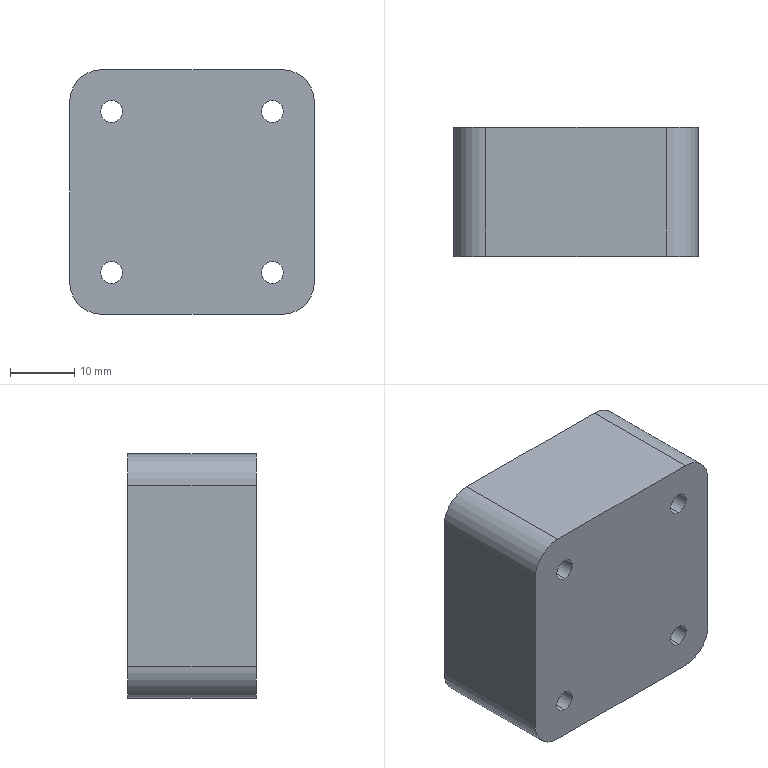Part | SolidWorks | features Extrusion 1, HoleWzd 1 | 1 solid | 30 faces | box 38 x 20 x 38 mm | volume 26957 mm3 | cylinder 20 | plane 10 | commonest cylinder face diameters 3.4 x8 6 x8 10 x4
STEP:
#1=CARTESIAN_POINT('',(-12.5,10.,-15.5));
#2=VERTEX_POINT('',#1);
#3=CARTESIAN_POINT('',(-12.5,10.,-9.5));
#4=VERTEX_POINT('',#3);
#5=CARTESIAN_POINT('',(-12.5,10.,-12.5));
#6=DIRECTION('',(0.,1.,0.));
#7=DIRECTION('',(0.,0.,1.));
#8=AXIS2_PLACEMENT_3D('',#5,#6,#7);
#9=CIRCLE('',#8,3.);
#10=EDGE_CURVE('',#2,#4,#9,.T.);
#11=ORIENTED_EDGE('',*,*,#10,.F.);
#12=CARTESIAN_POINT('',(-12.5,20.,-15.5));
#13=VERTEX_POINT('',#12);
#14=CARTESIAN_POINT('',(-12.5,20.,-15.5));
#15=DIRECTION('',(0.,1.,0.));
#16=VECTOR('',#15,1000.);
#17=LINE('',#14,#16);
#18=EDGE_CURVE('',#2,#13,#17,.T.);
#19=ORIENTED_EDGE('',*,*,#18,.T.);
#20=CARTESIAN_POINT('',(-12.5,20.,-9.5));
#21=VERTEX_POINT('',#20);
#22=CARTESIAN_POINT('',(-12.5,20.,-12.5));
#23=DIRECTION('',(0.,1.,0.));
#24=DIRECTION('',(0.,0.,1.));
#25=AXIS2_PLACEMENT_3D('',#22,#23,#24);
#26=CIRCLE('',#25,3.);
#27=EDGE_CURVE('',#13,#21,#26,.T.);
#28=ORIENTED_EDGE('',*,*,#27,.T.);
#29=CARTESIAN_POINT('',(-12.5,20.,-9.5));
#30=DIRECTION('',(0.,1.,0.));
#31=VECTOR('',#30,1000.);
#32=LINE('',#29,#31);
#33=EDGE_CURVE('',#4,#21,#32,.T.);
#34=ORIENTED_EDGE('',*,*,#33,.F.);
#35=EDGE_LOOP('',(#11,#19,#28,#34));
#36=FACE_OUTER_BOUND('',#35,.T.);
#37=CARTESIAN_POINT('',(-12.5,20.,-12.5));
#38=DIRECTION('',(0.,1.,0.));
#39=DIRECTION('',(0.,0.,1.));
#40=AXIS2_PLACEMENT_3D('',#37,#38,#39);
#41=CYLINDRICAL_SURFACE('',#40,3.);
#42=ADVANCED_FACE('',(#36),#41,.F.);
#43=CARTESIAN_POINT('',(-12.5,0.,-14.2));
#44=VERTEX_POINT('',#43);
#45=CARTESIAN_POINT('',(-12.5,0.,-10.8));
#46=VERTEX_POINT('',#45);
#47=CARTESIAN_POINT('',(-12.5,0.,-12.5));
#48=DIRECTION('',(0.,1.,0.));
#49=DIRECTION('',(0.,0.,1.));
#50=AXIS2_PLACEMENT_3D('',#47,#48,#49);
#51=CIRCLE('',#50,1.7);
#52=EDGE_CURVE('',#44,#46,#51,.T.);
#53=ORIENTED_EDGE('',*,*,#52,.F.);
#54=CARTESIAN_POINT('',(-12.5,10.,-14.2));
#55=VERTEX_POINT('',#54);
#56=CARTESIAN_POINT('',(-12.5,20.,-14.2));
#57=DIRECTION('',(0.,1.,0.));
#58=VECTOR('',#57,1000.);
#59=LINE('',#56,#58);
#60=EDGE_CURVE('',#44,#55,#59,.T.);
#61=ORIENTED_EDGE('',*,*,#60,.T.);
#62=CARTESIAN_POINT('',(-12.5,10.,-10.8));
#63=VERTEX_POINT('',#62);
#64=CARTESIAN_POINT('',(-12.5,10.,-12.5));
#65=DIRECTION('',(0.,1.,0.));
#66=DIRECTION('',(0.,0.,1.));
#67=AXIS2_PLACEMENT_3D('',#64,#65,#66);
#68=CIRCLE('',#67,1.7);
#69=EDGE_CURVE('',#55,#63,#68,.T.);
#70=ORIENTED_EDGE('',*,*,#69,.T.);
#71=CARTESIAN_POINT('',(-12.5,20.,-10.8));
#72=DIRECTION('',(0.,1.,0.));
#73=VECTOR('',#72,1000.);
#74=LINE('',#71,#73);
#75=EDGE_CURVE('',#46,#63,#74,.T.);
#76=ORIENTED_EDGE('',*,*,#75,.F.);
#77=EDGE_LOOP('',(#53,#61,#70,#76));
#78=FACE_OUTER_BOUND('',#77,.T.);
#79=CARTESIAN_POINT('',(-12.5,20.,-12.5));
#80=DIRECTION('',(0.,1.,0.));
#81=DIRECTION('',(0.,0.,1.));
#82=AXIS2_PLACEMENT_3D('',#79,#80,#81);
#83=CYLINDRICAL_SURFACE('',#82,1.7);
#84=ADVANCED_FACE('',(#78),#83,.F.);
#85=CARTESIAN_POINT('',(12.5,10.,-15.5));
#86=VERTEX_POINT('',#85);
#87=CARTESIAN_POINT('',(12.5,10.,-9.5));
#88=VERTEX_POINT('',#87);
#89=CARTESIAN_POINT('',(12.5,10.,-12.5));
#90=DIRECTION('',(0.,1.,0.));
#91=DIRECTION('',(0.,0.,1.));
#92=AXIS2_PLACEMENT_3D('',#89,#90,#91);
#93=CIRCLE('',#92,3.);
#94=EDGE_CURVE('',#86,#88,#93,.T.);
#95=ORIENTED_EDGE('',*,*,#94,.F.);
#96=CARTESIAN_POINT('',(12.5,20.,-15.5));
#97=VERTEX_POINT('',#96);
#98=CARTESIAN_POINT('',(12.5,20.,-15.5));
#99=DIRECTION('',(0.,1.,0.));
#100=VECTOR('',#99,1000.);
#101=LINE('',#98,#100);
#102=EDGE_CURVE('',#86,#97,#101,.T.);
#103=ORIENTED_EDGE('',*,*,#102,.T.);
#104=CARTESIAN_POINT('',(12.5,20.,-9.5));
#105=VERTEX_POINT('',#104);
#106=CARTESIAN_POINT('',(12.5,20.,-12.5));
#107=DIRECTION('',(0.,1.,0.));
#108=DIRECTION('',(0.,0.,1.));
#109=AXIS2_PLACEMENT_3D('',#106,#107,#108);
#110=CIRCLE('',#109,3.);
#111=EDGE_CURVE('',#97,#105,#110,.T.);
#112=ORIENTED_EDGE('',*,*,#111,.T.);
#113=CARTESIAN_POINT('',(12.5,20.,-9.5));
#114=DIRECTION('',(0.,1.,0.));
#115=VECTOR('',#114,1000.);
#116=LINE('',#113,#115);
#117=EDGE_CURVE('',#88,#105,#116,.T.);
#118=ORIENTED_EDGE('',*,*,#117,.F.);
#119=EDGE_LOOP('',(#95,#103,#112,#118));
#120=FACE_OUTER_BOUND('',#119,.T.);
#121=CARTESIAN_POINT('',(12.5,20.,-12.5));
#122=DIRECTION('',(0.,1.,0.));
#123=DIRECTION('',(0.,0.,1.));
#124=AXIS2_PLACEMENT_3D('',#121,#122,#123);
#125=CYLINDRICAL_SURFACE('',#124,3.);
#126=ADVANCED_FACE('',(#120),#125,.F.);
#127=CARTESIAN_POINT('',(12.5,0.,-14.2));
#128=VERTEX_POINT('',#127);
#129=CARTESIAN_POINT('',(12.5,0.,-10.8));
#130=VERTEX_POINT('',#129);
#131=CARTESIAN_POINT('',(12.5,0.,-12.5));
#132=DIRECTION('',(0.,1.,0.));
#133=DIRECTION('',(0.,0.,1.));
#134=AXIS2_PLACEMENT_3D('',#131,#132,#133);
#135=CIRCLE('',#134,1.7);
#136=EDGE_CURVE('',#128,#130,#135,.T.);
#137=ORIENTED_EDGE('',*,*,#136,.F.);
#138=CARTESIAN_POINT('',(12.5,10.,-14.2));
#139=VERTEX_POINT('',#138);
#140=CARTESIAN_POINT('',(12.5,20.,-14.2));
#141=DIRECTION('',(0.,1.,0.));
#142=VECTOR('',#141,1000.);
#143=LINE('',#140,#142);
#144=EDGE_CURVE('',#128,#139,#143,.T.);
#145=ORIENTED_EDGE('',*,*,#144,.T.);
#146=CARTESIAN_POINT('',(12.5,10.,-10.8));
#147=VERTEX_POINT('',#146);
#148=CARTESIAN_POINT('',(12.5,10.,-12.5));
#149=DIRECTION('',(0.,1.,0.));
#150=DIRECTION('',(0.,0.,1.));
#151=AXIS2_PLACEMENT_3D('',#148,#149,#150);
#152=CIRCLE('',#151,1.7);
#153=EDGE_CURVE('',#139,#147,#152,.T.);
#154=ORIENTED_EDGE('',*,*,#153,.T.);
#155=CARTESIAN_POINT('',(12.5,20.,-10.8));
#156=DIRECTION('',(0.,1.,0.));
#157=VECTOR('',#156,1000.);
#158=LINE('',#155,#157);
#159=EDGE_CURVE('',#130,#147,#158,.T.);
#160=ORIENTED_EDGE('',*,*,#159,.F.);
#161=EDGE_LOOP('',(#137,#145,#154,#160));
#162=FACE_OUTER_BOUND('',#161,.T.);
#163=CARTESIAN_POINT('',(12.5,20.,-12.5));
#164=DIRECTION('',(0.,1.,0.));
#165=DIRECTION('',(0.,0.,1.));
#166=AXIS2_PLACEMENT_3D('',#163,#164,#165);
#167=CYLINDRICAL_SURFACE('',#166,1.7);
#168=ADVANCED_FACE('',(#162),#167,.F.);
#169=CARTESIAN_POINT('',(12.5,10.,9.5));
#170=VERTEX_POINT('',#169);
#171=CARTESIAN_POINT('',(12.5,10.,15.5));
#172=VERTEX_POINT('',#171);
#173=CARTESIAN_POINT('',(12.5,10.,12.5));
#174=DIRECTION('',(0.,1.,0.));
#175=DIRECTION('',(0.,0.,1.));
#176=AXIS2_PLACEMENT_3D('',#173,#174,#175);
#177=CIRCLE('',#176,3.);
#178=EDGE_CURVE('',#170,#172,#177,.T.);
#179=ORIENTED_EDGE('',*,*,#178,.F.);
#180=CARTESIAN_POINT('',(12.5,20.,9.5));
#181=VERTEX_POINT('',#180);
#182=CARTESIAN_POINT('',(12.5,20.,9.5));
#183=DIRECTION('',(0.,1.,0.));
#184=VECTOR('',#183,1000.);
#185=LINE('',#182,#184);
#186=EDGE_CURVE('',#170,#181,#185,.T.);
#187=ORIENTED_EDGE('',*,*,#186,.T.);
#188=CARTESIAN_POINT('',(12.5,20.,15.5));
#189=VERTEX_POINT('',#188);
#190=CARTESIAN_POINT('',(12.5,20.,12.5));
#191=DIRECTION('',(0.,1.,0.));
#192=DIRECTION('',(0.,0.,1.));
#193=AXIS2_PLACEMENT_3D('',#190,#191,#192);
#194=CIRCLE('',#193,3.);
#195=EDGE_CURVE('',#181,#189,#194,.T.);
#196=ORIENTED_EDGE('',*,*,#195,.T.);
#197=CARTESIAN_POINT('',(12.5,20.,15.5));
#198=DIRECTION('',(0.,1.,0.));
#199=VECTOR('',#198,1000.);
#200=LINE('',#197,#199);
#201=EDGE_CURVE('',#172,#189,#200,.T.);
#202=ORIENTED_EDGE('',*,*,#201,.F.);
#203=EDGE_LOOP('',(#179,#187,#196,#202));
#204=FACE_OUTER_BOUND('',#203,.T.);
#205=CARTESIAN_POINT('',(12.5,20.,12.5));
#206=DIRECTION('',(0.,1.,0.));
#207=DIRECTION('',(0.,0.,1.));
#208=AXIS2_PLACEMENT_3D('',#205,#206,#207);
#209=CYLINDRICAL_SURFACE('',#208,3.);
#210=ADVANCED_FACE('',(#204),#209,.F.);
#211=CARTESIAN_POINT('',(12.5,0.,10.8));
#212=VERTEX_POINT('',#211);
#213=CARTESIAN_POINT('',(12.5,0.,14.2));
#214=VERTEX_POINT('',#213);
#215=CARTESIAN_POINT('',(12.5,0.,12.5));
#216=DIRECTION('',(0.,1.,0.));
#217=DIRECTION('',(0.,0.,1.));
#218=AXIS2_PLACEMENT_3D('',#215,#216,#217);
#219=CIRCLE('',#218,1.7);
#220=EDGE_CURVE('',#212,#214,#219,.T.);
#221=ORIENTED_EDGE('',*,*,#220,.F.);
#222=CARTESIAN_POINT('',(12.5,10.,10.8));
#223=VERTEX_POINT('',#222);
#224=CARTESIAN_POINT('',(12.5,20.,10.8));
#225=DIRECTION('',(0.,1.,0.));
#226=VECTOR('',#225,1000.);
#227=LINE('',#224,#226);
#228=EDGE_CURVE('',#212,#223,#227,.T.);
#229=ORIENTED_EDGE('',*,*,#228,.T.);
#230=CARTESIAN_POINT('',(12.5,10.,14.2));
#231=VERTEX_POINT('',#230);
#232=CARTESIAN_POINT('',(12.5,10.,12.5));
#233=DIRECTION('',(0.,1.,0.));
#234=DIRECTION('',(0.,0.,1.));
#235=AXIS2_PLACEMENT_3D('',#232,#233,#234);
#236=CIRCLE('',#235,1.7);
#237=EDGE_CURVE('',#223,#231,#236,.T.);
#238=ORIENTED_EDGE('',*,*,#237,.T.);
#239=CARTESIAN_POINT('',(12.5,20.,14.2));
#240=DIRECTION('',(0.,1.,0.));
#241=VECTOR('',#240,1000.);
#242=LINE('',#239,#241);
#243=EDGE_CURVE('',#214,#231,#242,.T.);
#244=ORIENTED_EDGE('',*,*,#243,.F.);
#245=EDGE_LOOP('',(#221,#229,#238,#244));
#246=FACE_OUTER_BOUND('',#245,.T.);
#247=CARTESIAN_POINT('',(12.5,20.,12.5));
#248=DIRECTION('',(0.,1.,0.));
#249=DIRECTION('',(0.,0.,1.));
#250=AXIS2_PLACEMENT_3D('',#247,#248,#249);
#251=CYLINDRICAL_SURFACE('',#250,1.7);
#252=ADVANCED_FACE('',(#246),#251,.F.);
#253=CARTESIAN_POINT('',(-12.5,10.,9.5));
#254=VERTEX_POINT('',#253);
#255=CARTESIAN_POINT('',(-12.5,10.,15.5));
#256=VERTEX_POINT('',#255);
#257=CARTESIAN_POINT('',(-12.5,10.,12.5));
#258=DIRECTION('',(0.,1.,0.));
#259=DIRECTION('',(0.,0.,1.));
#260=AXIS2_PLACEMENT_3D('',#257,#258,#259);
#261=CIRCLE('',#260,3.);
#262=EDGE_CURVE('',#254,#256,#261,.T.);
#263=ORIENTED_EDGE('',*,*,#262,.F.);
#264=CARTESIAN_POINT('',(-12.5,20.,9.5));
#265=VERTEX_POINT('',#264);
#266=CARTESIAN_POINT('',(-12.5,20.,9.5));
#267=DIRECTION('',(0.,1.,0.));
#268=VECTOR('',#267,1000.);
#269=LINE('',#266,#268);
#270=EDGE_CURVE('',#254,#265,#269,.T.);
#271=ORIENTED_EDGE('',*,*,#270,.T.);
#272=CARTESIAN_POINT('',(-12.5,20.,15.5));
#273=VERTEX_POINT('',#272);
#274=CARTESIAN_POINT('',(-12.5,20.,12.5));
#275=DIRECTION('',(0.,1.,0.));
#276=DIRECTION('',(0.,0.,1.));
#277=AXIS2_PLACEMENT_3D('',#274,#275,#276);
#278=CIRCLE('',#277,3.);
#279=EDGE_CURVE('',#265,#273,#278,.T.);
#280=ORIENTED_EDGE('',*,*,#279,.T.);
#281=CARTESIAN_POINT('',(-12.5,20.,15.5));
#282=DIRECTION('',(0.,1.,0.));
#283=VECTOR('',#282,1000.);
#284=LINE('',#281,#283);
#285=EDGE_CURVE('',#256,#273,#284,.T.);
#286=ORIENTED_EDGE('',*,*,#285,.F.);
#287=EDGE_LOOP('',(#263,#271,#280,#286));
#288=FACE_OUTER_BOUND('',#287,.T.);
#289=CARTESIAN_POINT('',(-12.5,20.,12.5));
#290=DIRECTION('',(0.,1.,0.));
#291=DIRECTION('',(0.,0.,1.));
#292=AXIS2_PLACEMENT_3D('',#289,#290,#291);
#293=CYLINDRICAL_SURFACE('',#292,3.);
#294=ADVANCED_FACE('',(#288),#293,.F.);
#295=CARTESIAN_POINT('',(-12.5,0.,10.8));
#296=VERTEX_POINT('',#295);
#297=CARTESIAN_POINT('',(-12.5,0.,14.2));
#298=VERTEX_POINT('',#297);
#299=CARTESIAN_POINT('',(-12.5,0.,12.5));
#300=DIRECTION('',(0.,1.,0.));
#301=DIRECTION('',(0.,0.,1.));
#302=AXIS2_PLACEMENT_3D('',#299,#300,#301);
#303=CIRCLE('',#302,1.7);
#304=EDGE_CURVE('',#296,#298,#303,.T.);
#305=ORIENTED_EDGE('',*,*,#304,.F.);
#306=CARTESIAN_POINT('',(-12.5,10.,10.8));
#307=VERTEX_POINT('',#306);
#308=CARTESIAN_POINT('',(-12.5,20.,10.8));
#309=DIRECTION('',(0.,1.,0.));
#310=VECTOR('',#309,1000.);
#311=LINE('',#308,#310);
#312=EDGE_CURVE('',#296,#307,#311,.T.);
#313=ORIENTED_EDGE('',*,*,#312,.T.);
#314=CARTESIAN_POINT('',(-12.5,10.,14.2));
#315=VERTEX_POINT('',#314);
#316=CARTESIAN_POINT('',(-12.5,10.,12.5));
#317=DIRECTION('',(0.,1.,0.));
#318=DIRECTION('',(0.,0.,1.));
#319=AXIS2_PLACEMENT_3D('',#316,#317,#318);
#320=CIRCLE('',#319,1.7);
#321=EDGE_CURVE('',#307,#315,#320,.T.);
#322=ORIENTED_EDGE('',*,*,#321,.T.);
#323=CARTESIAN_POINT('',(-12.5,20.,14.2));
#324=DIRECTION('',(0.,1.,0.));
#325=VECTOR('',#324,1000.);
#326=LINE('',#323,#325);
#327=EDGE_CURVE('',#298,#315,#326,.T.);
#328=ORIENTED_EDGE('',*,*,#327,.F.);
#329=EDGE_LOOP('',(#305,#313,#322,#328));
#330=FACE_OUTER_BOUND('',#329,.T.);
#331=CARTESIAN_POINT('',(-12.5,20.,12.5));
#332=DIRECTION('',(0.,1.,0.));
#333=DIRECTION('',(0.,0.,1.));
#334=AXIS2_PLACEMENT_3D('',#331,#332,#333);
#335=CYLINDRICAL_SURFACE('',#334,1.7);
#336=ADVANCED_FACE('',(#330),#335,.F.);
#337=CARTESIAN_POINT('',(19.,0.,-14.));
#338=VERTEX_POINT('',#337);
#339=CARTESIAN_POINT('',(14.,0.,-19.));
#340=VERTEX_POINT('',#339);
#341=CARTESIAN_POINT('',(14.,0.,-14.));
#342=DIRECTION('',(0.,1.,0.));
#343=DIRECTION('',(0.,0.,-1.));
#344=AXIS2_PLACEMENT_3D('',#341,#342,#343);
#345=CIRCLE('',#344,5.);
#346=EDGE_CURVE('',#338,#340,#345,.T.);
#347=ORIENTED_EDGE('',*,*,#346,.T.);
#348=CARTESIAN_POINT('',(14.,20.,-19.));
#349=VERTEX_POINT('',#348);
#350=CARTESIAN_POINT('',(14.,20.,-19.));
#351=DIRECTION('',(0.,-1.,0.));
#352=VECTOR('',#351,1000.);
#353=LINE('',#350,#352);
#354=EDGE_CURVE('',#349,#340,#353,.T.);
#355=ORIENTED_EDGE('',*,*,#354,.F.);
#356=CARTESIAN_POINT('',(19.,20.,-14.));
#357=VERTEX_POINT('',#356);
#358=CARTESIAN_POINT('',(14.,20.,-14.));
#359=DIRECTION('',(0.,1.,0.));
#360=DIRECTION('',(0.,0.,-1.));
#361=AXIS2_PLACEMENT_3D('',#358,#359,#360);
#362=CIRCLE('',#361,5.);
#363=EDGE_CURVE('',#357,#349,#362,.T.);
#364=ORIENTED_EDGE('',*,*,#363,.F.);
#365=CARTESIAN_POINT('',(19.,20.,-14.));
#366=DIRECTION('',(0.,-1.,0.));
#367=VECTOR('',#366,1000.);
#368=LINE('',#365,#367);
#369=EDGE_CURVE('',#357,#338,#368,.T.);
#370=ORIENTED_EDGE('',*,*,#369,.T.);
#371=EDGE_LOOP('',(#347,#355,#364,#370));
#372=FACE_OUTER_BOUND('',#371,.T.);
#373=CARTESIAN_POINT('',(14.,20.,-14.));
#374=DIRECTION('',(0.,-1.,0.));
#375=DIRECTION('',(0.,0.,-1.));
#376=AXIS2_PLACEMENT_3D('',#373,#374,#375);
#377=CYLINDRICAL_SURFACE('',#376,5.);
#378=ADVANCED_FACE('',(#372),#377,.T.);
#379=CARTESIAN_POINT('',(-14.,0.,-19.));
#380=VERTEX_POINT('',#379);
#381=CARTESIAN_POINT('',(-14.,0.,-19.));
#382=DIRECTION('',(-1.,0.,0.));
#383=VECTOR('',#382,1000.);
#384=LINE('',#381,#383);
#385=EDGE_CURVE('',#340,#380,#384,.T.);
#386=ORIENTED_EDGE('',*,*,#385,.T.);
#387=CARTESIAN_POINT('',(-14.,20.,-19.));
#388=VERTEX_POINT('',#387);
#389=CARTESIAN_POINT('',(-14.,20.,-19.));
#390=DIRECTION('',(0.,-1.,0.));
#391=VECTOR('',#390,1000.);
#392=LINE('',#389,#391);
#393=EDGE_CURVE('',#388,#380,#392,.T.);
#394=ORIENTED_EDGE('',*,*,#393,.F.);
#395=CARTESIAN_POINT('',(-14.,20.,-19.));
#396=DIRECTION('',(-1.,0.,0.));
#397=VECTOR('',#396,1000.);
#398=LINE('',#395,#397);
#399=EDGE_CURVE('',#349,#388,#398,.T.);
#400=ORIENTED_EDGE('',*,*,#399,.F.);
#401=ORIENTED_EDGE('',*,*,#354,.T.);
#402=EDGE_LOOP('',(#386,#394,#400,#401));
#403=FACE_OUTER_BOUND('',#402,.T.);
#404=CARTESIAN_POINT('',(-14.,20.,-19.));
#405=DIRECTION('',(0.,0.,1.));
#406=DIRECTION('',(1.,0.,0.));
#407=AXIS2_PLACEMENT_3D('',#404,#405,#406);
#408=PLANE('',#407);
#409=ADVANCED_FACE('',(#403),#408,.F.);
#410=CARTESIAN_POINT('',(-19.,0.,-14.));
#411=VERTEX_POINT('',#410);
#412=CARTESIAN_POINT('',(-14.,0.,-14.));
#413=DIRECTION('',(0.,1.,0.));
#414=DIRECTION('',(0.,0.,1.));
#415=AXIS2_PLACEMENT_3D('',#412,#413,#414);
#416=CIRCLE('',#415,5.);
#417=EDGE_CURVE('',#380,#411,#416,.T.);
#418=ORIENTED_EDGE('',*,*,#417,.T.);
#419=CARTESIAN_POINT('',(-19.,20.,-14.));
#420=VERTEX_POINT('',#419);
#421=CARTESIAN_POINT('',(-19.,20.,-14.));
#422=DIRECTION('',(0.,-1.,0.));
#423=VECTOR('',#422,1000.);
#424=LINE('',#421,#423);
#425=EDGE_CURVE('',#420,#411,#424,.T.);
#426=ORIENTED_EDGE('',*,*,#425,.F.);
#427=CARTESIAN_POINT('',(-14.,20.,-14.));
#428=DIRECTION('',(0.,1.,0.));
#429=DIRECTION('',(0.,0.,1.));
#430=AXIS2_PLACEMENT_3D('',#427,#428,#429);
#431=CIRCLE('',#430,5.);
#432=EDGE_CURVE('',#388,#420,#431,.T.);
#433=ORIENTED_EDGE('',*,*,#432,.F.);
#434=ORIENTED_EDGE('',*,*,#393,.T.);
#435=EDGE_LOOP('',(#418,#426,#433,#434));
#436=FACE_OUTER_BOUND('',#435,.T.);
#437=CARTESIAN_POINT('',(-14.,20.,-14.));
#438=DIRECTION('',(0.,-1.,0.));
#439=DIRECTION('',(0.,0.,-1.));
#440=AXIS2_PLACEMENT_3D('',#437,#438,#439);
#441=CYLINDRICAL_SURFACE('',#440,5.);
#442=ADVANCED_FACE('',(#436),#441,.T.);
#443=CARTESIAN_POINT('',(-19.,0.,14.));
#444=VERTEX_POINT('',#443);
#445=CARTESIAN_POINT('',(-19.,0.,-14.));
#446=DIRECTION('',(0.,0.,1.));
#447=VECTOR('',#446,1000.);
#448=LINE('',#445,#447);
#449=EDGE_CURVE('',#411,#444,#448,.T.);
#450=ORIENTED_EDGE('',*,*,#449,.T.);
#451=CARTESIAN_POINT('',(-19.,20.,14.));
#452=VERTEX_POINT('',#451);
#453=CARTESIAN_POINT('',(-19.,20.,14.));
#454=DIRECTION('',(0.,-1.,0.));
#455=VECTOR('',#454,1000.);
#456=LINE('',#453,#455);
#457=EDGE_CURVE('',#452,#444,#456,.T.);
#458=ORIENTED_EDGE('',*,*,#457,.F.);
#459=CARTESIAN_POINT('',(-19.,20.,-14.));
#460=DIRECTION('',(0.,0.,1.));
#461=VECTOR('',#460,1000.);
#462=LINE('',#459,#461);
#463=EDGE_CURVE('',#420,#452,#462,.T.);
#464=ORIENTED_EDGE('',*,*,#463,.F.);
#465=ORIENTED_EDGE('',*,*,#425,.T.);
#466=EDGE_LOOP('',(#450,#458,#464,#465));
#467=FACE_OUTER_BOUND('',#466,.T.);
#468=CARTESIAN_POINT('',(-19.,20.,-14.));
#469=DIRECTION('',(1.,0.,0.));
#470=DIRECTION('',(0.,0.,-1.));
#471=AXIS2_PLACEMENT_3D('',#468,#469,#470);
#472=PLANE('',#471);
#473=ADVANCED_FACE('',(#467),#472,.F.);
#474=CARTESIAN_POINT('',(-14.,0.,19.));
#475=VERTEX_POINT('',#474);
#476=CARTESIAN_POINT('',(-14.,0.,14.));
#477=DIRECTION('',(0.,1.,0.));
#478=DIRECTION('',(0.,0.,1.));
#479=AXIS2_PLACEMENT_3D('',#476,#477,#478);
#480=CIRCLE('',#479,5.);
#481=EDGE_CURVE('',#444,#475,#480,.T.);
#482=ORIENTED_EDGE('',*,*,#481,.T.);
#483=CARTESIAN_POINT('',(-14.,20.,19.));
#484=VERTEX_POINT('',#483);
#485=CARTESIAN_POINT('',(-14.,20.,19.));
#486=DIRECTION('',(0.,-1.,0.));
#487=VECTOR('',#486,1000.);
#488=LINE('',#485,#487);
#489=EDGE_CURVE('',#484,#475,#488,.T.);
#490=ORIENTED_EDGE('',*,*,#489,.F.);
#491=CARTESIAN_POINT('',(-14.,20.,14.));
#492=DIRECTION('',(0.,1.,0.));
#493=DIRECTION('',(0.,0.,1.));
#494=AXIS2_PLACEMENT_3D('',#491,#492,#493);
#495=CIRCLE('',#494,5.);
#496=EDGE_CURVE('',#452,#484,#495,.T.);
#497=ORIENTED_EDGE('',*,*,#496,.F.);
#498=ORIENTED_EDGE('',*,*,#457,.T.);
#499=EDGE_LOOP('',(#482,#490,#497,#498));
#500=FACE_OUTER_BOUND('',#499,.T.);
#501=CARTESIAN_POINT('',(-14.,20.,14.));
#502=DIRECTION('',(0.,-1.,0.));
#503=DIRECTION('',(0.,0.,-1.));
#504=AXIS2_PLACEMENT_3D('',#501,#502,#503);
#505=CYLINDRICAL_SURFACE('',#504,5.);
#506=ADVANCED_FACE('',(#500),#505,.T.);
#507=CARTESIAN_POINT('',(14.,0.,19.));
#508=VERTEX_POINT('',#507);
#509=CARTESIAN_POINT('',(-14.,0.,19.));
#510=DIRECTION('',(1.,0.,0.));
#511=VECTOR('',#510,1000.);
#512=LINE('',#509,#511);
#513=EDGE_CURVE('',#475,#508,#512,.T.);
#514=ORIENTED_EDGE('',*,*,#513,.T.);
#515=CARTESIAN_POINT('',(14.,20.,19.));
#516=VERTEX_POINT('',#515);
#517=CARTESIAN_POINT('',(14.,20.,19.));
#518=DIRECTION('',(0.,-1.,0.));
#519=VECTOR('',#518,1000.);
#520=LINE('',#517,#519);
#521=EDGE_CURVE('',#516,#508,#520,.T.);
#522=ORIENTED_EDGE('',*,*,#521,.F.);
#523=CARTESIAN_POINT('',(-14.,20.,19.));
#524=DIRECTION('',(1.,0.,0.));
#525=VECTOR('',#524,1000.);
#526=LINE('',#523,#525);
#527=EDGE_CURVE('',#484,#516,#526,.T.);
#528=ORIENTED_EDGE('',*,*,#527,.F.);
#529=ORIENTED_EDGE('',*,*,#489,.T.);
#530=EDGE_LOOP('',(#514,#522,#528,#529));
#531=FACE_OUTER_BOUND('',#530,.T.);
#532=CARTESIAN_POINT('',(-14.,20.,19.));
#533=DIRECTION('',(0.,0.,-1.));
#534=DIRECTION('',(-1.,0.,0.));
#535=AXIS2_PLACEMENT_3D('',#532,#533,#534);
#536=PLANE('',#535);
#537=ADVANCED_FACE('',(#531),#536,.F.);
#538=CARTESIAN_POINT('',(19.,0.,14.));
#539=VERTEX_POINT('',#538);
#540=CARTESIAN_POINT('',(14.,0.,14.));
#541=DIRECTION('',(0.,1.,0.));
#542=DIRECTION('',(0.,0.,1.));
#543=AXIS2_PLACEMENT_3D('',#540,#541,#542);
#544=CIRCLE('',#543,5.);
#545=EDGE_CURVE('',#508,#539,#544,.T.);
#546=ORIENTED_EDGE('',*,*,#545,.T.);
#547=CARTESIAN_POINT('',(19.,20.,14.));
#548=VERTEX_POINT('',#547);
#549=CARTESIAN_POINT('',(19.,20.,14.));
#550=DIRECTION('',(0.,-1.,0.));
#551=VECTOR('',#550,1000.);
#552=LINE('',#549,#551);
#553=EDGE_CURVE('',#548,#539,#552,.T.);
#554=ORIENTED_EDGE('',*,*,#553,.F.);
#555=CARTESIAN_POINT('',(14.,20.,14.));
#556=DIRECTION('',(0.,1.,0.));
#557=DIRECTION('',(0.,0.,1.));
#558=AXIS2_PLACEMENT_3D('',#555,#556,#557);
#559=CIRCLE('',#558,5.);
#560=EDGE_CURVE('',#516,#548,#559,.T.);
#561=ORIENTED_EDGE('',*,*,#560,.F.);
#562=ORIENTED_EDGE('',*,*,#521,.T.);
#563=EDGE_LOOP('',(#546,#554,#561,#562));
#564=FACE_OUTER_BOUND('',#563,.T.);
#565=CARTESIAN_POINT('',(14.,20.,14.));
#566=DIRECTION('',(0.,-1.,0.));
#567=DIRECTION('',(0.,0.,-1.));
#568=AXIS2_PLACEMENT_3D('',#565,#566,#567);
#569=CYLINDRICAL_SURFACE('',#568,5.);
#570=ADVANCED_FACE('',(#564),#569,.T.);
#571=CARTESIAN_POINT('',(19.,0.,-14.));
#572=DIRECTION('',(0.,0.,-1.));
#573=VECTOR('',#572,1000.);
#574=LINE('',#571,#573);
#575=EDGE_CURVE('',#539,#338,#574,.T.);
#576=ORIENTED_EDGE('',*,*,#575,.T.);
#577=ORIENTED_EDGE('',*,*,#369,.F.);
#578=CARTESIAN_POINT('',(19.,20.,-14.));
#579=DIRECTION('',(0.,0.,-1.));
#580=VECTOR('',#579,1000.);
#581=LINE('',#578,#580);
#582=EDGE_CURVE('',#548,#357,#581,.T.);
#583=ORIENTED_EDGE('',*,*,#582,.F.);
#584=ORIENTED_EDGE('',*,*,#553,.T.);
#585=EDGE_LOOP('',(#576,#577,#583,#584));
#586=FACE_OUTER_BOUND('',#585,.T.);
#587=CARTESIAN_POINT('',(19.,20.,-14.));
#588=DIRECTION('',(-1.,0.,0.));
#589=DIRECTION('',(0.,0.,1.));
#590=AXIS2_PLACEMENT_3D('',#587,#588,#589);
#591=PLANE('',#590);
#592=ADVANCED_FACE('',(#586),#591,.F.);
#593=CARTESIAN_POINT('',(-12.5,20.,-12.5));
#594=DIRECTION('',(0.,1.,0.));
#595=DIRECTION('',(0.,0.,1.));
#596=AXIS2_PLACEMENT_3D('',#593,#594,#595);
#597=CIRCLE('',#596,3.);
#598=EDGE_CURVE('',#21,#13,#597,.T.);
#599=ORIENTED_EDGE('',*,*,#598,.F.);
#600=ORIENTED_EDGE('',*,*,#27,.F.);
#601=EDGE_LOOP('',(#599,#600));
#602=FACE_BOUND('',#601,.T.);
#603=CARTESIAN_POINT('',(12.5,20.,-12.5));
#604=DIRECTION('',(0.,1.,0.));
#605=DIRECTION('',(0.,0.,1.));
#606=AXIS2_PLACEMENT_3D('',#603,#604,#605);
#607=CIRCLE('',#606,3.);
#608=EDGE_CURVE('',#105,#97,#607,.T.);
#609=ORIENTED_EDGE('',*,*,#608,.F.);
#610=ORIENTED_EDGE('',*,*,#111,.F.);
#611=EDGE_LOOP('',(#609,#610));
#612=FACE_BOUND('',#611,.T.);
#613=CARTESIAN_POINT('',(12.5,20.,12.5));
#614=DIRECTION('',(0.,1.,0.));
#615=DIRECTION('',(0.,0.,1.));
#616=AXIS2_PLACEMENT_3D('',#613,#614,#615);
#617=CIRCLE('',#616,3.);
#618=EDGE_CURVE('',#189,#181,#617,.T.);
#619=ORIENTED_EDGE('',*,*,#618,.F.);
#620=ORIENTED_EDGE('',*,*,#195,.F.);
#621=EDGE_LOOP('',(#619,#620));
#622=FACE_BOUND('',#621,.T.);
#623=CARTESIAN_POINT('',(-12.5,20.,12.5));
#624=DIRECTION('',(0.,1.,0.));
#625=DIRECTION('',(0.,0.,1.));
#626=AXIS2_PLACEMENT_3D('',#623,#624,#625);
#627=CIRCLE('',#626,3.);
#628=EDGE_CURVE('',#273,#265,#627,.T.);
#629=ORIENTED_EDGE('',*,*,#628,.F.);
#630=ORIENTED_EDGE('',*,*,#279,.F.);
#631=EDGE_LOOP('',(#629,#630));
#632=FACE_BOUND('',#631,.T.);
#633=ORIENTED_EDGE('',*,*,#363,.T.);
#634=ORIENTED_EDGE('',*,*,#399,.T.);
#635=ORIENTED_EDGE('',*,*,#432,.T.);
#636=ORIENTED_EDGE('',*,*,#463,.T.);
#637=ORIENTED_EDGE('',*,*,#496,.T.);
#638=ORIENTED_EDGE('',*,*,#527,.T.);
#639=ORIENTED_EDGE('',*,*,#560,.T.);
#640=ORIENTED_EDGE('',*,*,#582,.T.);
#641=EDGE_LOOP('',(#633,#634,#635,#636,#637,#638,#639,#640));
#642=FACE_OUTER_BOUND('',#641,.T.);
#643=CARTESIAN_POINT('',(14.,20.,-14.));
#644=DIRECTION('',(0.,-1.,0.));
#645=DIRECTION('',(0.,0.,-1.));
#646=AXIS2_PLACEMENT_3D('',#643,#644,#645);
#647=PLANE('',#646);
#648=ADVANCED_FACE('',(#602,#612,#622,#632,#642),#647,.F.);
#649=CARTESIAN_POINT('',(-12.5,0.,-12.5));
#650=DIRECTION('',(0.,1.,0.));
#651=DIRECTION('',(0.,0.,1.));
#652=AXIS2_PLACEMENT_3D('',#649,#650,#651);
#653=CIRCLE('',#652,1.7);
#654=EDGE_CURVE('',#46,#44,#653,.T.);
#655=ORIENTED_EDGE('',*,*,#654,.T.);
#656=ORIENTED_EDGE('',*,*,#52,.T.);
#657=EDGE_LOOP('',(#655,#656));
#658=FACE_BOUND('',#657,.T.);
#659=CARTESIAN_POINT('',(12.5,0.,-12.5));
#660=DIRECTION('',(0.,1.,0.));
#661=DIRECTION('',(0.,0.,1.));
#662=AXIS2_PLACEMENT_3D('',#659,#660,#661);
#663=CIRCLE('',#662,1.7);
#664=EDGE_CURVE('',#130,#128,#663,.T.);
#665=ORIENTED_EDGE('',*,*,#664,.T.);
#666=ORIENTED_EDGE('',*,*,#136,.T.);
#667=EDGE_LOOP('',(#665,#666));
#668=FACE_BOUND('',#667,.T.);
#669=CARTESIAN_POINT('',(12.5,0.,12.5));
#670=DIRECTION('',(0.,1.,0.));
#671=DIRECTION('',(0.,0.,1.));
#672=AXIS2_PLACEMENT_3D('',#669,#670,#671);
#673=CIRCLE('',#672,1.7);
#674=EDGE_CURVE('',#214,#212,#673,.T.);
#675=ORIENTED_EDGE('',*,*,#674,.T.);
#676=ORIENTED_EDGE('',*,*,#220,.T.);
#677=EDGE_LOOP('',(#675,#676));
#678=FACE_BOUND('',#677,.T.);
#679=CARTESIAN_POINT('',(-12.5,0.,12.5));
#680=DIRECTION('',(0.,1.,0.));
#681=DIRECTION('',(0.,0.,1.));
#682=AXIS2_PLACEMENT_3D('',#679,#680,#681);
#683=CIRCLE('',#682,1.7);
#684=EDGE_CURVE('',#298,#296,#683,.T.);
#685=ORIENTED_EDGE('',*,*,#684,.T.);
#686=ORIENTED_EDGE('',*,*,#304,.T.);
#687=EDGE_LOOP('',(#685,#686));
#688=FACE_BOUND('',#687,.T.);
#689=ORIENTED_EDGE('',*,*,#346,.F.);
#690=ORIENTED_EDGE('',*,*,#575,.F.);
#691=ORIENTED_EDGE('',*,*,#545,.F.);
#692=ORIENTED_EDGE('',*,*,#513,.F.);
#693=ORIENTED_EDGE('',*,*,#481,.F.);
#694=ORIENTED_EDGE('',*,*,#449,.F.);
#695=ORIENTED_EDGE('',*,*,#417,.F.);
#696=ORIENTED_EDGE('',*,*,#385,.F.);
#697=EDGE_LOOP('',(#689,#690,#691,#692,#693,#694,#695,#696));
#698=FACE_OUTER_BOUND('',#697,.T.);
#699=CARTESIAN_POINT('',(14.,0.,-14.));
#700=DIRECTION('',(0.,-1.,0.));
#701=DIRECTION('',(0.,0.,-1.));
#702=AXIS2_PLACEMENT_3D('',#699,#700,#701);
#703=PLANE('',#702);
#704=ADVANCED_FACE('',(#658,#668,#678,#688,#698),#703,.T.);
#705=ORIENTED_EDGE('',*,*,#312,.F.);
#706=ORIENTED_EDGE('',*,*,#684,.F.);
#707=ORIENTED_EDGE('',*,*,#327,.T.);
#708=CARTESIAN_POINT('',(-12.5,10.,12.5));
#709=DIRECTION('',(0.,1.,0.));
#710=DIRECTION('',(0.,0.,1.));
#711=AXIS2_PLACEMENT_3D('',#708,#709,#710);
#712=CIRCLE('',#711,1.7);
#713=EDGE_CURVE('',#315,#307,#712,.T.);
#714=ORIENTED_EDGE('',*,*,#713,.T.);
#715=EDGE_LOOP('',(#705,#706,#707,#714));
#716=FACE_OUTER_BOUND('',#715,.T.);
#717=CARTESIAN_POINT('',(-12.5,20.,12.5));
#718=DIRECTION('',(0.,1.,0.));
#719=DIRECTION('',(0.,0.,1.));
#720=AXIS2_PLACEMENT_3D('',#717,#718,#719);
#721=CYLINDRICAL_SURFACE('',#720,1.7);
#722=ADVANCED_FACE('',(#716),#721,.F.);
#723=ORIENTED_EDGE('',*,*,#713,.F.);
#724=ORIENTED_EDGE('',*,*,#321,.F.);
#725=EDGE_LOOP('',(#723,#724));
#726=FACE_BOUND('',#725,.T.);
#727=CARTESIAN_POINT('',(-12.5,10.,12.5));
#728=DIRECTION('',(0.,1.,0.));
#729=DIRECTION('',(0.,0.,1.));
#730=AXIS2_PLACEMENT_3D('',#727,#728,#729);
#731=CIRCLE('',#730,3.);
#732=EDGE_CURVE('',#256,#254,#731,.T.);
#733=ORIENTED_EDGE('',*,*,#732,.T.);
#734=ORIENTED_EDGE('',*,*,#262,.T.);
#735=EDGE_LOOP('',(#733,#734));
#736=FACE_OUTER_BOUND('',#735,.T.);
#737=CARTESIAN_POINT('',(-10.8,10.,12.5));
#738=DIRECTION('',(0.,-1.,0.));
#739=DIRECTION('',(0.,0.,-1.));
#740=AXIS2_PLACEMENT_3D('',#737,#738,#739);
#741=PLANE('',#740);
#742=ADVANCED_FACE('',(#726,#736),#741,.F.);
#743=ORIENTED_EDGE('',*,*,#270,.F.);
#744=ORIENTED_EDGE('',*,*,#732,.F.);
#745=ORIENTED_EDGE('',*,*,#285,.T.);
#746=ORIENTED_EDGE('',*,*,#628,.T.);
#747=EDGE_LOOP('',(#743,#744,#745,#746));
#748=FACE_OUTER_BOUND('',#747,.T.);
#749=CARTESIAN_POINT('',(-12.5,20.,12.5));
#750=DIRECTION('',(0.,1.,0.));
#751=DIRECTION('',(0.,0.,1.));
#752=AXIS2_PLACEMENT_3D('',#749,#750,#751);
#753=CYLINDRICAL_SURFACE('',#752,3.);
#754=ADVANCED_FACE('',(#748),#753,.F.);
#755=ORIENTED_EDGE('',*,*,#228,.F.);
#756=ORIENTED_EDGE('',*,*,#674,.F.);
#757=ORIENTED_EDGE('',*,*,#243,.T.);
#758=CARTESIAN_POINT('',(12.5,10.,12.5));
#759=DIRECTION('',(0.,1.,0.));
#760=DIRECTION('',(0.,0.,1.));
#761=AXIS2_PLACEMENT_3D('',#758,#759,#760);
#762=CIRCLE('',#761,1.7);
#763=EDGE_CURVE('',#231,#223,#762,.T.);
#764=ORIENTED_EDGE('',*,*,#763,.T.);
#765=EDGE_LOOP('',(#755,#756,#757,#764));
#766=FACE_OUTER_BOUND('',#765,.T.);
#767=CARTESIAN_POINT('',(12.5,20.,12.5));
#768=DIRECTION('',(0.,1.,0.));
#769=DIRECTION('',(0.,0.,1.));
#770=AXIS2_PLACEMENT_3D('',#767,#768,#769);
#771=CYLINDRICAL_SURFACE('',#770,1.7);
#772=ADVANCED_FACE('',(#766),#771,.F.);
#773=ORIENTED_EDGE('',*,*,#763,.F.);
#774=ORIENTED_EDGE('',*,*,#237,.F.);
#775=EDGE_LOOP('',(#773,#774));
#776=FACE_BOUND('',#775,.T.);
#777=CARTESIAN_POINT('',(12.5,10.,12.5));
#778=DIRECTION('',(0.,1.,0.));
#779=DIRECTION('',(0.,0.,1.));
#780=AXIS2_PLACEMENT_3D('',#777,#778,#779);
#781=CIRCLE('',#780,3.);
#782=EDGE_CURVE('',#172,#170,#781,.T.);
#783=ORIENTED_EDGE('',*,*,#782,.T.);
#784=ORIENTED_EDGE('',*,*,#178,.T.);
#785=EDGE_LOOP('',(#783,#784));
#786=FACE_OUTER_BOUND('',#785,.T.);
#787=CARTESIAN_POINT('',(14.2,10.,12.5));
#788=DIRECTION('',(0.,-1.,0.));
#789=DIRECTION('',(0.,0.,-1.));
#790=AXIS2_PLACEMENT_3D('',#787,#788,#789);
#791=PLANE('',#790);
#792=ADVANCED_FACE('',(#776,#786),#791,.F.);
#793=ORIENTED_EDGE('',*,*,#186,.F.);
#794=ORIENTED_EDGE('',*,*,#782,.F.);
#795=ORIENTED_EDGE('',*,*,#201,.T.);
#796=ORIENTED_EDGE('',*,*,#618,.T.);
#797=EDGE_LOOP('',(#793,#794,#795,#796));
#798=FACE_OUTER_BOUND('',#797,.T.);
#799=CARTESIAN_POINT('',(12.5,20.,12.5));
#800=DIRECTION('',(0.,1.,0.));
#801=DIRECTION('',(0.,0.,1.));
#802=AXIS2_PLACEMENT_3D('',#799,#800,#801);
#803=CYLINDRICAL_SURFACE('',#802,3.);
#804=ADVANCED_FACE('',(#798),#803,.F.);
#805=ORIENTED_EDGE('',*,*,#144,.F.);
#806=ORIENTED_EDGE('',*,*,#664,.F.);
#807=ORIENTED_EDGE('',*,*,#159,.T.);
#808=CARTESIAN_POINT('',(12.5,10.,-12.5));
#809=DIRECTION('',(0.,1.,0.));
#810=DIRECTION('',(0.,0.,1.));
#811=AXIS2_PLACEMENT_3D('',#808,#809,#810);
#812=CIRCLE('',#811,1.7);
#813=EDGE_CURVE('',#147,#139,#812,.T.);
#814=ORIENTED_EDGE('',*,*,#813,.T.);
#815=EDGE_LOOP('',(#805,#806,#807,#814));
#816=FACE_OUTER_BOUND('',#815,.T.);
#817=CARTESIAN_POINT('',(12.5,20.,-12.5));
#818=DIRECTION('',(0.,1.,0.));
#819=DIRECTION('',(0.,0.,1.));
#820=AXIS2_PLACEMENT_3D('',#817,#818,#819);
#821=CYLINDRICAL_SURFACE('',#820,1.7);
#822=ADVANCED_FACE('',(#816),#821,.F.);
#823=ORIENTED_EDGE('',*,*,#813,.F.);
#824=ORIENTED_EDGE('',*,*,#153,.F.);
#825=EDGE_LOOP('',(#823,#824));
#826=FACE_BOUND('',#825,.T.);
#827=CARTESIAN_POINT('',(12.5,10.,-12.5));
#828=DIRECTION('',(0.,1.,0.));
#829=DIRECTION('',(0.,0.,1.));
#830=AXIS2_PLACEMENT_3D('',#827,#828,#829);
#831=CIRCLE('',#830,3.);
#832=EDGE_CURVE('',#88,#86,#831,.T.);
#833=ORIENTED_EDGE('',*,*,#832,.T.);
#834=ORIENTED_EDGE('',*,*,#94,.T.);
#835=EDGE_LOOP('',(#833,#834));
#836=FACE_OUTER_BOUND('',#835,.T.);
#837=CARTESIAN_POINT('',(14.2,10.,-12.5));
#838=DIRECTION('',(0.,-1.,0.));
#839=DIRECTION('',(0.,0.,-1.));
#840=AXIS2_PLACEMENT_3D('',#837,#838,#839);
#841=PLANE('',#840);
#842=ADVANCED_FACE('',(#826,#836),#841,.F.);
#843=ORIENTED_EDGE('',*,*,#102,.F.);
#844=ORIENTED_EDGE('',*,*,#832,.F.);
#845=ORIENTED_EDGE('',*,*,#117,.T.);
#846=ORIENTED_EDGE('',*,*,#608,.T.);
#847=EDGE_LOOP('',(#843,#844,#845,#846));
#848=FACE_OUTER_BOUND('',#847,.T.);
#849=CARTESIAN_POINT('',(12.5,20.,-12.5));
#850=DIRECTION('',(0.,1.,0.));
#851=DIRECTION('',(0.,0.,1.));
#852=AXIS2_PLACEMENT_3D('',#849,#850,#851);
#853=CYLINDRICAL_SURFACE('',#852,3.);
#854=ADVANCED_FACE('',(#848),#853,.F.);
#855=ORIENTED_EDGE('',*,*,#60,.F.);
#856=ORIENTED_EDGE('',*,*,#654,.F.);
#857=ORIENTED_EDGE('',*,*,#75,.T.);
#858=CARTESIAN_POINT('',(-12.5,10.,-12.5));
#859=DIRECTION('',(0.,1.,0.));
#860=DIRECTION('',(0.,0.,1.));
#861=AXIS2_PLACEMENT_3D('',#858,#859,#860);
#862=CIRCLE('',#861,1.7);
#863=EDGE_CURVE('',#63,#55,#862,.T.);
#864=ORIENTED_EDGE('',*,*,#863,.T.);
#865=EDGE_LOOP('',(#855,#856,#857,#864));
#866=FACE_OUTER_BOUND('',#865,.T.);
#867=CARTESIAN_POINT('',(-12.5,20.,-12.5));
#868=DIRECTION('',(0.,1.,0.));
#869=DIRECTION('',(0.,0.,1.));
#870=AXIS2_PLACEMENT_3D('',#867,#868,#869);
#871=CYLINDRICAL_SURFACE('',#870,1.7);
#872=ADVANCED_FACE('',(#866),#871,.F.);
#873=ORIENTED_EDGE('',*,*,#863,.F.);
#874=ORIENTED_EDGE('',*,*,#69,.F.);
#875=EDGE_LOOP('',(#873,#874));
#876=FACE_BOUND('',#875,.T.);
#877=CARTESIAN_POINT('',(-12.5,10.,-12.5));
#878=DIRECTION('',(0.,1.,0.));
#879=DIRECTION('',(0.,0.,1.));
#880=AXIS2_PLACEMENT_3D('',#877,#878,#879);
#881=CIRCLE('',#880,3.);
#882=EDGE_CURVE('',#4,#2,#881,.T.);
#883=ORIENTED_EDGE('',*,*,#882,.T.);
#884=ORIENTED_EDGE('',*,*,#10,.T.);
#885=EDGE_LOOP('',(#883,#884));
#886=FACE_OUTER_BOUND('',#885,.T.);
#887=CARTESIAN_POINT('',(-10.8,10.,-12.5));
#888=DIRECTION('',(0.,-1.,0.));
#889=DIRECTION('',(0.,0.,-1.));
#890=AXIS2_PLACEMENT_3D('',#887,#888,#889);
#891=PLANE('',#890);
#892=ADVANCED_FACE('',(#876,#886),#891,.F.);
#893=ORIENTED_EDGE('',*,*,#18,.F.);
#894=ORIENTED_EDGE('',*,*,#882,.F.);
#895=ORIENTED_EDGE('',*,*,#33,.T.);
#896=ORIENTED_EDGE('',*,*,#598,.T.);
#897=EDGE_LOOP('',(#893,#894,#895,#896));
#898=FACE_OUTER_BOUND('',#897,.T.);
#899=CARTESIAN_POINT('',(-12.5,20.,-12.5));
#900=DIRECTION('',(0.,1.,0.));
#901=DIRECTION('',(0.,0.,1.));
#902=AXIS2_PLACEMENT_3D('',#899,#900,#901);
#903=CYLINDRICAL_SURFACE('',#902,3.);
#904=ADVANCED_FACE('',(#898),#903,.F.);
#905=CLOSED_SHELL('',(#42,#84,#126,#168,#210,#252,#294,#336,#378,#409,#442,#473,#506,#537,#570,#592,#648,#704,#722,#742,#754,#772,#792,#804,#822,#842,#854,#872,#892,#904));
#906=MANIFOLD_SOLID_BREP('',#905);
#907=CARTESIAN_POINT('',(0.,0.,0.));
#908=DIRECTION('',(0.,0.,1.));
#909=DIRECTION('',(1.,0.,0.));
#910=AXIS2_PLACEMENT_3D('',#907,#908,#909);
#911=(LENGTH_UNIT()NAMED_UNIT(*)SI_UNIT(.MILLI.,.METRE.));
#912=UNCERTAINTY_MEASURE_WITH_UNIT(LENGTH_MEASURE(0.00001),#911,'','');
#913=(NAMED_UNIT(*)PLANE_ANGLE_UNIT()SI_UNIT($,.RADIAN.));
#914=(NAMED_UNIT(*)SI_UNIT($,.STERADIAN.)SOLID_ANGLE_UNIT());
#915=(GEOMETRIC_REPRESENTATION_CONTEXT(3)GLOBAL_UNCERTAINTY_ASSIGNED_CONTEXT((#912))GLOBAL_UNIT_ASSIGNED_CONTEXT((#911,#913,#914))REPRESENTATION_CONTEXT('',''));
#916=ADVANCED_BREP_SHAPE_REPRESENTATION('',(#906,#910),#915);